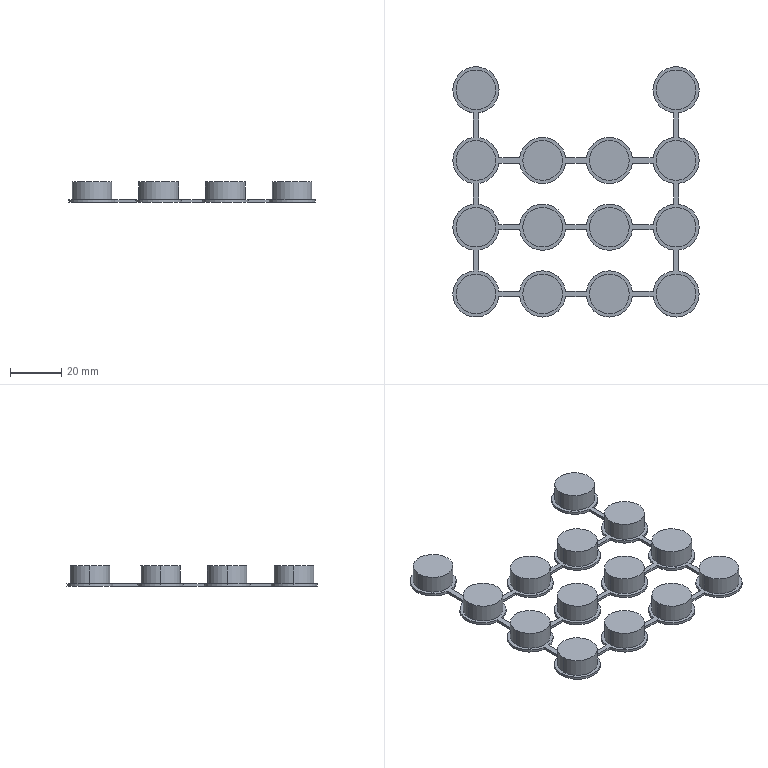Part | SolidWorks | features Extrusion 1, ICE 1 | 1 solid | 111 faces | box 96 x 97.5 x 8 mm | volume 22308 mm3 | cylinder 65 | plane 46 | commonest cylinder face diameters 18 x37 15.5 x28